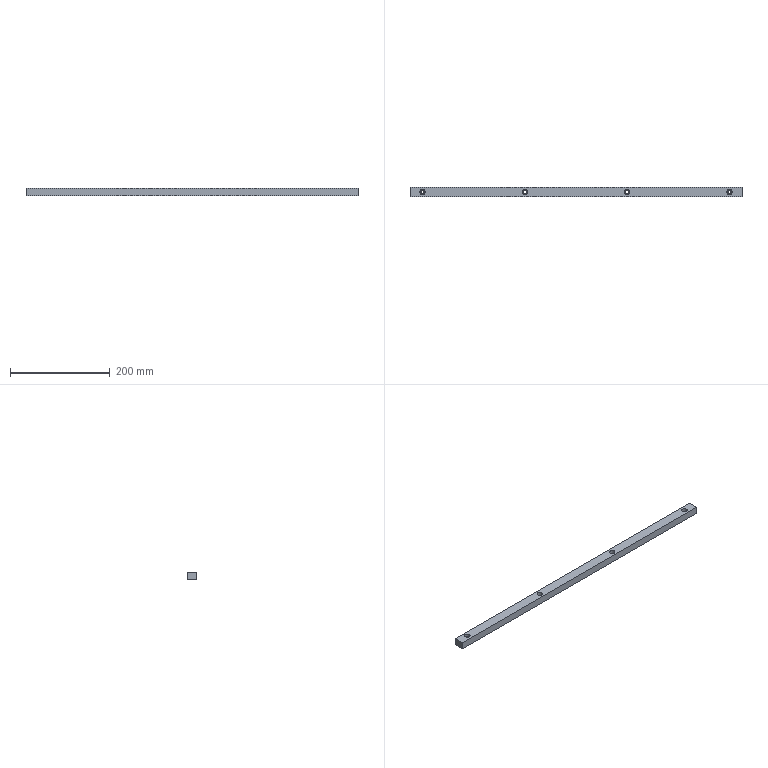Part | SolidWorks | features Extrusion 1, HoleWzd 1 | 1 solid | 26 faces | box 665 x 20 x 15 mm | volume 195793 mm3 | cylinder 16 | plane 10 | commonest cylinder face diameters 6.6 x8 11 x8
STEP:
#1=CARTESIAN_POINT('',(-313.,0.,8.2));
#2=VERTEX_POINT('',#1);
#3=CARTESIAN_POINT('',(-302.,0.,8.2));
#4=VERTEX_POINT('',#3);
#5=CARTESIAN_POINT('',(-307.5,0.,8.2));
#6=DIRECTION('',(0.,0.,1.));
#7=DIRECTION('',(1.,0.,0.));
#8=AXIS2_PLACEMENT_3D('',#5,#6,#7);
#9=CIRCLE('',#8,5.5);
#10=EDGE_CURVE('',#2,#4,#9,.T.);
#11=ORIENTED_EDGE('',*,*,#10,.F.);
#12=CARTESIAN_POINT('',(-313.,0.,15.));
#13=VERTEX_POINT('',#12);
#14=CARTESIAN_POINT('',(-313.,0.,15.));
#15=DIRECTION('',(0.,0.,1.));
#16=VECTOR('',#15,1000.);
#17=LINE('',#14,#16);
#18=EDGE_CURVE('',#2,#13,#17,.T.);
#19=ORIENTED_EDGE('',*,*,#18,.T.);
#20=CARTESIAN_POINT('',(-302.,0.,15.));
#21=VERTEX_POINT('',#20);
#22=CARTESIAN_POINT('',(-307.5,0.,15.));
#23=DIRECTION('',(0.,0.,1.));
#24=DIRECTION('',(1.,0.,0.));
#25=AXIS2_PLACEMENT_3D('',#22,#23,#24);
#26=CIRCLE('',#25,5.5);
#27=EDGE_CURVE('',#13,#21,#26,.T.);
#28=ORIENTED_EDGE('',*,*,#27,.T.);
#29=CARTESIAN_POINT('',(-302.,0.,15.));
#30=DIRECTION('',(0.,0.,1.));
#31=VECTOR('',#30,1000.);
#32=LINE('',#29,#31);
#33=EDGE_CURVE('',#4,#21,#32,.T.);
#34=ORIENTED_EDGE('',*,*,#33,.F.);
#35=EDGE_LOOP('',(#11,#19,#28,#34));
#36=FACE_OUTER_BOUND('',#35,.T.);
#37=CARTESIAN_POINT('',(-307.5,0.,15.));
#38=DIRECTION('',(0.,0.,1.));
#39=DIRECTION('',(1.,0.,0.));
#40=AXIS2_PLACEMENT_3D('',#37,#38,#39);
#41=CYLINDRICAL_SURFACE('',#40,5.5);
#42=ADVANCED_FACE('',(#36),#41,.F.);
#43=CARTESIAN_POINT('',(-310.8,0.,0.));
#44=VERTEX_POINT('',#43);
#45=CARTESIAN_POINT('',(-304.2,0.,0.));
#46=VERTEX_POINT('',#45);
#47=CARTESIAN_POINT('',(-307.5,0.,0.));
#48=DIRECTION('',(0.,0.,1.));
#49=DIRECTION('',(1.,0.,0.));
#50=AXIS2_PLACEMENT_3D('',#47,#48,#49);
#51=CIRCLE('',#50,3.3);
#52=EDGE_CURVE('',#44,#46,#51,.T.);
#53=ORIENTED_EDGE('',*,*,#52,.F.);
#54=CARTESIAN_POINT('',(-310.8,0.,8.2));
#55=VERTEX_POINT('',#54);
#56=CARTESIAN_POINT('',(-310.8,0.,15.));
#57=DIRECTION('',(0.,0.,1.));
#58=VECTOR('',#57,1000.);
#59=LINE('',#56,#58);
#60=EDGE_CURVE('',#44,#55,#59,.T.);
#61=ORIENTED_EDGE('',*,*,#60,.T.);
#62=CARTESIAN_POINT('',(-304.2,0.,8.2));
#63=VERTEX_POINT('',#62);
#64=CARTESIAN_POINT('',(-307.5,0.,8.2));
#65=DIRECTION('',(0.,0.,1.));
#66=DIRECTION('',(1.,0.,0.));
#67=AXIS2_PLACEMENT_3D('',#64,#65,#66);
#68=CIRCLE('',#67,3.3);
#69=EDGE_CURVE('',#55,#63,#68,.T.);
#70=ORIENTED_EDGE('',*,*,#69,.T.);
#71=CARTESIAN_POINT('',(-304.2,0.,15.));
#72=DIRECTION('',(0.,0.,1.));
#73=VECTOR('',#72,1000.);
#74=LINE('',#71,#73);
#75=EDGE_CURVE('',#46,#63,#74,.T.);
#76=ORIENTED_EDGE('',*,*,#75,.F.);
#77=EDGE_LOOP('',(#53,#61,#70,#76));
#78=FACE_OUTER_BOUND('',#77,.T.);
#79=CARTESIAN_POINT('',(-307.5,0.,15.));
#80=DIRECTION('',(0.,0.,1.));
#81=DIRECTION('',(1.,0.,0.));
#82=AXIS2_PLACEMENT_3D('',#79,#80,#81);
#83=CYLINDRICAL_SURFACE('',#82,3.3);
#84=ADVANCED_FACE('',(#78),#83,.F.);
#85=CARTESIAN_POINT('',(302.,0.,8.2));
#86=VERTEX_POINT('',#85);
#87=CARTESIAN_POINT('',(313.,0.,8.2));
#88=VERTEX_POINT('',#87);
#89=CARTESIAN_POINT('',(307.5,0.,8.2));
#90=DIRECTION('',(0.,0.,1.));
#91=DIRECTION('',(1.,0.,0.));
#92=AXIS2_PLACEMENT_3D('',#89,#90,#91);
#93=CIRCLE('',#92,5.5);
#94=EDGE_CURVE('',#86,#88,#93,.T.);
#95=ORIENTED_EDGE('',*,*,#94,.F.);
#96=CARTESIAN_POINT('',(302.,0.,15.));
#97=VERTEX_POINT('',#96);
#98=CARTESIAN_POINT('',(302.,0.,15.));
#99=DIRECTION('',(0.,0.,1.));
#100=VECTOR('',#99,1000.);
#101=LINE('',#98,#100);
#102=EDGE_CURVE('',#86,#97,#101,.T.);
#103=ORIENTED_EDGE('',*,*,#102,.T.);
#104=CARTESIAN_POINT('',(313.,0.,15.));
#105=VERTEX_POINT('',#104);
#106=CARTESIAN_POINT('',(307.5,0.,15.));
#107=DIRECTION('',(0.,0.,1.));
#108=DIRECTION('',(1.,0.,0.));
#109=AXIS2_PLACEMENT_3D('',#106,#107,#108);
#110=CIRCLE('',#109,5.5);
#111=EDGE_CURVE('',#97,#105,#110,.T.);
#112=ORIENTED_EDGE('',*,*,#111,.T.);
#113=CARTESIAN_POINT('',(313.,0.,15.));
#114=DIRECTION('',(0.,0.,1.));
#115=VECTOR('',#114,1000.);
#116=LINE('',#113,#115);
#117=EDGE_CURVE('',#88,#105,#116,.T.);
#118=ORIENTED_EDGE('',*,*,#117,.F.);
#119=EDGE_LOOP('',(#95,#103,#112,#118));
#120=FACE_OUTER_BOUND('',#119,.T.);
#121=CARTESIAN_POINT('',(307.5,0.,15.));
#122=DIRECTION('',(0.,0.,1.));
#123=DIRECTION('',(1.,0.,0.));
#124=AXIS2_PLACEMENT_3D('',#121,#122,#123);
#125=CYLINDRICAL_SURFACE('',#124,5.5);
#126=ADVANCED_FACE('',(#120),#125,.F.);
#127=CARTESIAN_POINT('',(304.2,0.,0.));
#128=VERTEX_POINT('',#127);
#129=CARTESIAN_POINT('',(310.8,0.,0.));
#130=VERTEX_POINT('',#129);
#131=CARTESIAN_POINT('',(307.5,0.,0.));
#132=DIRECTION('',(0.,0.,1.));
#133=DIRECTION('',(1.,0.,0.));
#134=AXIS2_PLACEMENT_3D('',#131,#132,#133);
#135=CIRCLE('',#134,3.3);
#136=EDGE_CURVE('',#128,#130,#135,.T.);
#137=ORIENTED_EDGE('',*,*,#136,.F.);
#138=CARTESIAN_POINT('',(304.2,0.,8.2));
#139=VERTEX_POINT('',#138);
#140=CARTESIAN_POINT('',(304.2,0.,15.));
#141=DIRECTION('',(0.,0.,1.));
#142=VECTOR('',#141,1000.);
#143=LINE('',#140,#142);
#144=EDGE_CURVE('',#128,#139,#143,.T.);
#145=ORIENTED_EDGE('',*,*,#144,.T.);
#146=CARTESIAN_POINT('',(310.8,0.,8.2));
#147=VERTEX_POINT('',#146);
#148=CARTESIAN_POINT('',(307.5,0.,8.2));
#149=DIRECTION('',(0.,0.,1.));
#150=DIRECTION('',(1.,0.,0.));
#151=AXIS2_PLACEMENT_3D('',#148,#149,#150);
#152=CIRCLE('',#151,3.3);
#153=EDGE_CURVE('',#139,#147,#152,.T.);
#154=ORIENTED_EDGE('',*,*,#153,.T.);
#155=CARTESIAN_POINT('',(310.8,0.,15.));
#156=DIRECTION('',(0.,0.,1.));
#157=VECTOR('',#156,1000.);
#158=LINE('',#155,#157);
#159=EDGE_CURVE('',#130,#147,#158,.T.);
#160=ORIENTED_EDGE('',*,*,#159,.F.);
#161=EDGE_LOOP('',(#137,#145,#154,#160));
#162=FACE_OUTER_BOUND('',#161,.T.);
#163=CARTESIAN_POINT('',(307.5,0.,15.));
#164=DIRECTION('',(0.,0.,1.));
#165=DIRECTION('',(1.,0.,0.));
#166=AXIS2_PLACEMENT_3D('',#163,#164,#165);
#167=CYLINDRICAL_SURFACE('',#166,3.3);
#168=ADVANCED_FACE('',(#162),#167,.F.);
#169=CARTESIAN_POINT('',(-108.,0.,8.2));
#170=VERTEX_POINT('',#169);
#171=CARTESIAN_POINT('',(-97.,0.,8.2));
#172=VERTEX_POINT('',#171);
#173=CARTESIAN_POINT('',(-102.5,0.,8.2));
#174=DIRECTION('',(0.,0.,1.));
#175=DIRECTION('',(1.,0.,0.));
#176=AXIS2_PLACEMENT_3D('',#173,#174,#175);
#177=CIRCLE('',#176,5.5);
#178=EDGE_CURVE('',#170,#172,#177,.T.);
#179=ORIENTED_EDGE('',*,*,#178,.F.);
#180=CARTESIAN_POINT('',(-108.,0.,15.));
#181=VERTEX_POINT('',#180);
#182=CARTESIAN_POINT('',(-108.,0.,15.));
#183=DIRECTION('',(0.,0.,1.));
#184=VECTOR('',#183,1000.);
#185=LINE('',#182,#184);
#186=EDGE_CURVE('',#170,#181,#185,.T.);
#187=ORIENTED_EDGE('',*,*,#186,.T.);
#188=CARTESIAN_POINT('',(-97.,0.,15.));
#189=VERTEX_POINT('',#188);
#190=CARTESIAN_POINT('',(-102.5,0.,15.));
#191=DIRECTION('',(0.,0.,1.));
#192=DIRECTION('',(1.,0.,0.));
#193=AXIS2_PLACEMENT_3D('',#190,#191,#192);
#194=CIRCLE('',#193,5.5);
#195=EDGE_CURVE('',#181,#189,#194,.T.);
#196=ORIENTED_EDGE('',*,*,#195,.T.);
#197=CARTESIAN_POINT('',(-97.,0.,15.));
#198=DIRECTION('',(0.,0.,1.));
#199=VECTOR('',#198,1000.);
#200=LINE('',#197,#199);
#201=EDGE_CURVE('',#172,#189,#200,.T.);
#202=ORIENTED_EDGE('',*,*,#201,.F.);
#203=EDGE_LOOP('',(#179,#187,#196,#202));
#204=FACE_OUTER_BOUND('',#203,.T.);
#205=CARTESIAN_POINT('',(-102.5,0.,15.));
#206=DIRECTION('',(0.,0.,1.));
#207=DIRECTION('',(1.,0.,0.));
#208=AXIS2_PLACEMENT_3D('',#205,#206,#207);
#209=CYLINDRICAL_SURFACE('',#208,5.5);
#210=ADVANCED_FACE('',(#204),#209,.F.);
#211=CARTESIAN_POINT('',(-105.8,0.,0.));
#212=VERTEX_POINT('',#211);
#213=CARTESIAN_POINT('',(-99.2,0.,0.));
#214=VERTEX_POINT('',#213);
#215=CARTESIAN_POINT('',(-102.5,0.,0.));
#216=DIRECTION('',(0.,0.,1.));
#217=DIRECTION('',(1.,0.,0.));
#218=AXIS2_PLACEMENT_3D('',#215,#216,#217);
#219=CIRCLE('',#218,3.3);
#220=EDGE_CURVE('',#212,#214,#219,.T.);
#221=ORIENTED_EDGE('',*,*,#220,.F.);
#222=CARTESIAN_POINT('',(-105.8,0.,8.2));
#223=VERTEX_POINT('',#222);
#224=CARTESIAN_POINT('',(-105.8,0.,15.));
#225=DIRECTION('',(0.,0.,1.));
#226=VECTOR('',#225,1000.);
#227=LINE('',#224,#226);
#228=EDGE_CURVE('',#212,#223,#227,.T.);
#229=ORIENTED_EDGE('',*,*,#228,.T.);
#230=CARTESIAN_POINT('',(-99.2,0.,8.2));
#231=VERTEX_POINT('',#230);
#232=CARTESIAN_POINT('',(-102.5,0.,8.2));
#233=DIRECTION('',(0.,0.,1.));
#234=DIRECTION('',(1.,0.,0.));
#235=AXIS2_PLACEMENT_3D('',#232,#233,#234);
#236=CIRCLE('',#235,3.3);
#237=EDGE_CURVE('',#223,#231,#236,.T.);
#238=ORIENTED_EDGE('',*,*,#237,.T.);
#239=CARTESIAN_POINT('',(-99.2,0.,15.));
#240=DIRECTION('',(0.,0.,1.));
#241=VECTOR('',#240,1000.);
#242=LINE('',#239,#241);
#243=EDGE_CURVE('',#214,#231,#242,.T.);
#244=ORIENTED_EDGE('',*,*,#243,.F.);
#245=EDGE_LOOP('',(#221,#229,#238,#244));
#246=FACE_OUTER_BOUND('',#245,.T.);
#247=CARTESIAN_POINT('',(-102.5,0.,15.));
#248=DIRECTION('',(0.,0.,1.));
#249=DIRECTION('',(1.,0.,0.));
#250=AXIS2_PLACEMENT_3D('',#247,#248,#249);
#251=CYLINDRICAL_SURFACE('',#250,3.3);
#252=ADVANCED_FACE('',(#246),#251,.F.);
#253=CARTESIAN_POINT('',(97.,0.,8.2));
#254=VERTEX_POINT('',#253);
#255=CARTESIAN_POINT('',(108.,0.,8.2));
#256=VERTEX_POINT('',#255);
#257=CARTESIAN_POINT('',(102.5,0.,8.2));
#258=DIRECTION('',(0.,0.,1.));
#259=DIRECTION('',(1.,0.,0.));
#260=AXIS2_PLACEMENT_3D('',#257,#258,#259);
#261=CIRCLE('',#260,5.5);
#262=EDGE_CURVE('',#254,#256,#261,.T.);
#263=ORIENTED_EDGE('',*,*,#262,.F.);
#264=CARTESIAN_POINT('',(97.,0.,15.));
#265=VERTEX_POINT('',#264);
#266=CARTESIAN_POINT('',(97.,0.,15.));
#267=DIRECTION('',(0.,0.,1.));
#268=VECTOR('',#267,1000.);
#269=LINE('',#266,#268);
#270=EDGE_CURVE('',#254,#265,#269,.T.);
#271=ORIENTED_EDGE('',*,*,#270,.T.);
#272=CARTESIAN_POINT('',(108.,0.,15.));
#273=VERTEX_POINT('',#272);
#274=CARTESIAN_POINT('',(102.5,0.,15.));
#275=DIRECTION('',(0.,0.,1.));
#276=DIRECTION('',(1.,0.,0.));
#277=AXIS2_PLACEMENT_3D('',#274,#275,#276);
#278=CIRCLE('',#277,5.5);
#279=EDGE_CURVE('',#265,#273,#278,.T.);
#280=ORIENTED_EDGE('',*,*,#279,.T.);
#281=CARTESIAN_POINT('',(108.,0.,15.));
#282=DIRECTION('',(0.,0.,1.));
#283=VECTOR('',#282,1000.);
#284=LINE('',#281,#283);
#285=EDGE_CURVE('',#256,#273,#284,.T.);
#286=ORIENTED_EDGE('',*,*,#285,.F.);
#287=EDGE_LOOP('',(#263,#271,#280,#286));
#288=FACE_OUTER_BOUND('',#287,.T.);
#289=CARTESIAN_POINT('',(102.5,0.,15.));
#290=DIRECTION('',(0.,0.,1.));
#291=DIRECTION('',(1.,0.,0.));
#292=AXIS2_PLACEMENT_3D('',#289,#290,#291);
#293=CYLINDRICAL_SURFACE('',#292,5.5);
#294=ADVANCED_FACE('',(#288),#293,.F.);
#295=CARTESIAN_POINT('',(99.2,0.,0.));
#296=VERTEX_POINT('',#295);
#297=CARTESIAN_POINT('',(105.8,0.,0.));
#298=VERTEX_POINT('',#297);
#299=CARTESIAN_POINT('',(102.5,0.,0.));
#300=DIRECTION('',(0.,0.,1.));
#301=DIRECTION('',(1.,0.,0.));
#302=AXIS2_PLACEMENT_3D('',#299,#300,#301);
#303=CIRCLE('',#302,3.3);
#304=EDGE_CURVE('',#296,#298,#303,.T.);
#305=ORIENTED_EDGE('',*,*,#304,.F.);
#306=CARTESIAN_POINT('',(99.2,0.,8.2));
#307=VERTEX_POINT('',#306);
#308=CARTESIAN_POINT('',(99.2,0.,15.));
#309=DIRECTION('',(0.,0.,1.));
#310=VECTOR('',#309,1000.);
#311=LINE('',#308,#310);
#312=EDGE_CURVE('',#296,#307,#311,.T.);
#313=ORIENTED_EDGE('',*,*,#312,.T.);
#314=CARTESIAN_POINT('',(105.8,0.,8.2));
#315=VERTEX_POINT('',#314);
#316=CARTESIAN_POINT('',(102.5,0.,8.2));
#317=DIRECTION('',(0.,0.,1.));
#318=DIRECTION('',(1.,0.,0.));
#319=AXIS2_PLACEMENT_3D('',#316,#317,#318);
#320=CIRCLE('',#319,3.3);
#321=EDGE_CURVE('',#307,#315,#320,.T.);
#322=ORIENTED_EDGE('',*,*,#321,.T.);
#323=CARTESIAN_POINT('',(105.8,0.,15.));
#324=DIRECTION('',(0.,0.,1.));
#325=VECTOR('',#324,1000.);
#326=LINE('',#323,#325);
#327=EDGE_CURVE('',#298,#315,#326,.T.);
#328=ORIENTED_EDGE('',*,*,#327,.F.);
#329=EDGE_LOOP('',(#305,#313,#322,#328));
#330=FACE_OUTER_BOUND('',#329,.T.);
#331=CARTESIAN_POINT('',(102.5,0.,15.));
#332=DIRECTION('',(0.,0.,1.));
#333=DIRECTION('',(1.,0.,0.));
#334=AXIS2_PLACEMENT_3D('',#331,#332,#333);
#335=CYLINDRICAL_SURFACE('',#334,3.3);
#336=ADVANCED_FACE('',(#330),#335,.F.);
#337=CARTESIAN_POINT('',(332.5,-10.,0.));
#338=VERTEX_POINT('',#337);
#339=CARTESIAN_POINT('',(332.5,10.,0.));
#340=VERTEX_POINT('',#339);
#341=CARTESIAN_POINT('',(332.5,10.,0.));
#342=DIRECTION('',(0.,1.,0.));
#343=VECTOR('',#342,1000.);
#344=LINE('',#341,#343);
#345=EDGE_CURVE('',#338,#340,#344,.T.);
#346=ORIENTED_EDGE('',*,*,#345,.T.);
#347=CARTESIAN_POINT('',(332.5,10.,15.));
#348=VERTEX_POINT('',#347);
#349=CARTESIAN_POINT('',(332.5,10.,15.));
#350=DIRECTION('',(0.,0.,-1.));
#351=VECTOR('',#350,1000.);
#352=LINE('',#349,#351);
#353=EDGE_CURVE('',#348,#340,#352,.T.);
#354=ORIENTED_EDGE('',*,*,#353,.F.);
#355=CARTESIAN_POINT('',(332.5,-10.,15.));
#356=VERTEX_POINT('',#355);
#357=CARTESIAN_POINT('',(332.5,10.,15.));
#358=DIRECTION('',(0.,1.,0.));
#359=VECTOR('',#358,1000.);
#360=LINE('',#357,#359);
#361=EDGE_CURVE('',#356,#348,#360,.T.);
#362=ORIENTED_EDGE('',*,*,#361,.F.);
#363=CARTESIAN_POINT('',(332.5,-10.,15.));
#364=DIRECTION('',(0.,0.,-1.));
#365=VECTOR('',#364,1000.);
#366=LINE('',#363,#365);
#367=EDGE_CURVE('',#356,#338,#366,.T.);
#368=ORIENTED_EDGE('',*,*,#367,.T.);
#369=EDGE_LOOP('',(#346,#354,#362,#368));
#370=FACE_OUTER_BOUND('',#369,.T.);
#371=CARTESIAN_POINT('',(332.5,10.,15.));
#372=DIRECTION('',(-1.,0.,0.));
#373=DIRECTION('',(0.,0.,1.));
#374=AXIS2_PLACEMENT_3D('',#371,#372,#373);
#375=PLANE('',#374);
#376=ADVANCED_FACE('',(#370),#375,.F.);
#377=CARTESIAN_POINT('',(-332.5,10.,0.));
#378=VERTEX_POINT('',#377);
#379=CARTESIAN_POINT('',(-332.5,10.,0.));
#380=DIRECTION('',(-1.,0.,0.));
#381=VECTOR('',#380,1000.);
#382=LINE('',#379,#381);
#383=EDGE_CURVE('',#340,#378,#382,.T.);
#384=ORIENTED_EDGE('',*,*,#383,.T.);
#385=CARTESIAN_POINT('',(-332.5,10.,15.));
#386=VERTEX_POINT('',#385);
#387=CARTESIAN_POINT('',(-332.5,10.,15.));
#388=DIRECTION('',(0.,0.,-1.));
#389=VECTOR('',#388,1000.);
#390=LINE('',#387,#389);
#391=EDGE_CURVE('',#386,#378,#390,.T.);
#392=ORIENTED_EDGE('',*,*,#391,.F.);
#393=CARTESIAN_POINT('',(-332.5,10.,15.));
#394=DIRECTION('',(-1.,0.,0.));
#395=VECTOR('',#394,1000.);
#396=LINE('',#393,#395);
#397=EDGE_CURVE('',#348,#386,#396,.T.);
#398=ORIENTED_EDGE('',*,*,#397,.F.);
#399=ORIENTED_EDGE('',*,*,#353,.T.);
#400=EDGE_LOOP('',(#384,#392,#398,#399));
#401=FACE_OUTER_BOUND('',#400,.T.);
#402=CARTESIAN_POINT('',(-332.5,10.,15.));
#403=DIRECTION('',(0.,-1.,0.));
#404=DIRECTION('',(0.,0.,-1.));
#405=AXIS2_PLACEMENT_3D('',#402,#403,#404);
#406=PLANE('',#405);
#407=ADVANCED_FACE('',(#401),#406,.F.);
#408=CARTESIAN_POINT('',(-332.5,-10.,0.));
#409=VERTEX_POINT('',#408);
#410=CARTESIAN_POINT('',(-332.5,10.,0.));
#411=DIRECTION('',(0.,-1.,0.));
#412=VECTOR('',#411,1000.);
#413=LINE('',#410,#412);
#414=EDGE_CURVE('',#378,#409,#413,.T.);
#415=ORIENTED_EDGE('',*,*,#414,.T.);
#416=CARTESIAN_POINT('',(-332.5,-10.,15.));
#417=VERTEX_POINT('',#416);
#418=CARTESIAN_POINT('',(-332.5,-10.,15.));
#419=DIRECTION('',(0.,0.,-1.));
#420=VECTOR('',#419,1000.);
#421=LINE('',#418,#420);
#422=EDGE_CURVE('',#417,#409,#421,.T.);
#423=ORIENTED_EDGE('',*,*,#422,.F.);
#424=CARTESIAN_POINT('',(-332.5,10.,15.));
#425=DIRECTION('',(0.,-1.,0.));
#426=VECTOR('',#425,1000.);
#427=LINE('',#424,#426);
#428=EDGE_CURVE('',#386,#417,#427,.T.);
#429=ORIENTED_EDGE('',*,*,#428,.F.);
#430=ORIENTED_EDGE('',*,*,#391,.T.);
#431=EDGE_LOOP('',(#415,#423,#429,#430));
#432=FACE_OUTER_BOUND('',#431,.T.);
#433=CARTESIAN_POINT('',(-332.5,10.,15.));
#434=DIRECTION('',(1.,0.,0.));
#435=DIRECTION('',(0.,0.,-1.));
#436=AXIS2_PLACEMENT_3D('',#433,#434,#435);
#437=PLANE('',#436);
#438=ADVANCED_FACE('',(#432),#437,.F.);
#439=CARTESIAN_POINT('',(-332.5,-10.,0.));
#440=DIRECTION('',(1.,0.,0.));
#441=VECTOR('',#440,1000.);
#442=LINE('',#439,#441);
#443=EDGE_CURVE('',#409,#338,#442,.T.);
#444=ORIENTED_EDGE('',*,*,#443,.T.);
#445=ORIENTED_EDGE('',*,*,#367,.F.);
#446=CARTESIAN_POINT('',(-332.5,-10.,15.));
#447=DIRECTION('',(1.,0.,0.));
#448=VECTOR('',#447,1000.);
#449=LINE('',#446,#448);
#450=EDGE_CURVE('',#417,#356,#449,.T.);
#451=ORIENTED_EDGE('',*,*,#450,.F.);
#452=ORIENTED_EDGE('',*,*,#422,.T.);
#453=EDGE_LOOP('',(#444,#445,#451,#452));
#454=FACE_OUTER_BOUND('',#453,.T.);
#455=CARTESIAN_POINT('',(-332.5,-10.,15.));
#456=DIRECTION('',(0.,1.,0.));
#457=DIRECTION('',(0.,0.,1.));
#458=AXIS2_PLACEMENT_3D('',#455,#456,#457);
#459=PLANE('',#458);
#460=ADVANCED_FACE('',(#454),#459,.F.);
#461=CARTESIAN_POINT('',(-307.5,0.,15.));
#462=DIRECTION('',(0.,0.,1.));
#463=DIRECTION('',(1.,0.,0.));
#464=AXIS2_PLACEMENT_3D('',#461,#462,#463);
#465=CIRCLE('',#464,5.5);
#466=EDGE_CURVE('',#21,#13,#465,.T.);
#467=ORIENTED_EDGE('',*,*,#466,.F.);
#468=ORIENTED_EDGE('',*,*,#27,.F.);
#469=EDGE_LOOP('',(#467,#468));
#470=FACE_BOUND('',#469,.T.);
#471=CARTESIAN_POINT('',(307.5,0.,15.));
#472=DIRECTION('',(0.,0.,1.));
#473=DIRECTION('',(1.,0.,0.));
#474=AXIS2_PLACEMENT_3D('',#471,#472,#473);
#475=CIRCLE('',#474,5.5);
#476=EDGE_CURVE('',#105,#97,#475,.T.);
#477=ORIENTED_EDGE('',*,*,#476,.F.);
#478=ORIENTED_EDGE('',*,*,#111,.F.);
#479=EDGE_LOOP('',(#477,#478));
#480=FACE_BOUND('',#479,.T.);
#481=CARTESIAN_POINT('',(-102.5,0.,15.));
#482=DIRECTION('',(0.,0.,1.));
#483=DIRECTION('',(1.,0.,0.));
#484=AXIS2_PLACEMENT_3D('',#481,#482,#483);
#485=CIRCLE('',#484,5.5);
#486=EDGE_CURVE('',#189,#181,#485,.T.);
#487=ORIENTED_EDGE('',*,*,#486,.F.);
#488=ORIENTED_EDGE('',*,*,#195,.F.);
#489=EDGE_LOOP('',(#487,#488));
#490=FACE_BOUND('',#489,.T.);
#491=CARTESIAN_POINT('',(102.5,0.,15.));
#492=DIRECTION('',(0.,0.,1.));
#493=DIRECTION('',(1.,0.,0.));
#494=AXIS2_PLACEMENT_3D('',#491,#492,#493);
#495=CIRCLE('',#494,5.5);
#496=EDGE_CURVE('',#273,#265,#495,.T.);
#497=ORIENTED_EDGE('',*,*,#496,.F.);
#498=ORIENTED_EDGE('',*,*,#279,.F.);
#499=EDGE_LOOP('',(#497,#498));
#500=FACE_BOUND('',#499,.T.);
#501=ORIENTED_EDGE('',*,*,#361,.T.);
#502=ORIENTED_EDGE('',*,*,#397,.T.);
#503=ORIENTED_EDGE('',*,*,#428,.T.);
#504=ORIENTED_EDGE('',*,*,#450,.T.);
#505=EDGE_LOOP('',(#501,#502,#503,#504));
#506=FACE_OUTER_BOUND('',#505,.T.);
#507=CARTESIAN_POINT('',(0.,0.,15.));
#508=DIRECTION('',(0.,0.,1.));
#509=DIRECTION('',(1.,0.,0.));
#510=AXIS2_PLACEMENT_3D('',#507,#508,#509);
#511=PLANE('',#510);
#512=ADVANCED_FACE('',(#470,#480,#490,#500,#506),#511,.T.);
#513=CARTESIAN_POINT('',(-307.5,0.,0.));
#514=DIRECTION('',(0.,0.,1.));
#515=DIRECTION('',(1.,0.,0.));
#516=AXIS2_PLACEMENT_3D('',#513,#514,#515);
#517=CIRCLE('',#516,3.3);
#518=EDGE_CURVE('',#46,#44,#517,.T.);
#519=ORIENTED_EDGE('',*,*,#518,.T.);
#520=ORIENTED_EDGE('',*,*,#52,.T.);
#521=EDGE_LOOP('',(#519,#520));
#522=FACE_BOUND('',#521,.T.);
#523=CARTESIAN_POINT('',(307.5,0.,0.));
#524=DIRECTION('',(0.,0.,1.));
#525=DIRECTION('',(1.,0.,0.));
#526=AXIS2_PLACEMENT_3D('',#523,#524,#525);
#527=CIRCLE('',#526,3.3);
#528=EDGE_CURVE('',#130,#128,#527,.T.);
#529=ORIENTED_EDGE('',*,*,#528,.T.);
#530=ORIENTED_EDGE('',*,*,#136,.T.);
#531=EDGE_LOOP('',(#529,#530));
#532=FACE_BOUND('',#531,.T.);
#533=CARTESIAN_POINT('',(-102.5,0.,0.));
#534=DIRECTION('',(0.,0.,1.));
#535=DIRECTION('',(1.,0.,0.));
#536=AXIS2_PLACEMENT_3D('',#533,#534,#535);
#537=CIRCLE('',#536,3.3);
#538=EDGE_CURVE('',#214,#212,#537,.T.);
#539=ORIENTED_EDGE('',*,*,#538,.T.);
#540=ORIENTED_EDGE('',*,*,#220,.T.);
#541=EDGE_LOOP('',(#539,#540));
#542=FACE_BOUND('',#541,.T.);
#543=CARTESIAN_POINT('',(102.5,0.,0.));
#544=DIRECTION('',(0.,0.,1.));
#545=DIRECTION('',(1.,0.,0.));
#546=AXIS2_PLACEMENT_3D('',#543,#544,#545);
#547=CIRCLE('',#546,3.3);
#548=EDGE_CURVE('',#298,#296,#547,.T.);
#549=ORIENTED_EDGE('',*,*,#548,.T.);
#550=ORIENTED_EDGE('',*,*,#304,.T.);
#551=EDGE_LOOP('',(#549,#550));
#552=FACE_BOUND('',#551,.T.);
#553=ORIENTED_EDGE('',*,*,#345,.F.);
#554=ORIENTED_EDGE('',*,*,#443,.F.);
#555=ORIENTED_EDGE('',*,*,#414,.F.);
#556=ORIENTED_EDGE('',*,*,#383,.F.);
#557=EDGE_LOOP('',(#553,#554,#555,#556));
#558=FACE_OUTER_BOUND('',#557,.T.);
#559=CARTESIAN_POINT('',(0.,0.,0.));
#560=DIRECTION('',(0.,0.,1.));
#561=DIRECTION('',(1.,0.,0.));
#562=AXIS2_PLACEMENT_3D('',#559,#560,#561);
#563=PLANE('',#562);
#564=ADVANCED_FACE('',(#522,#532,#542,#552,#558),#563,.F.);
#565=ORIENTED_EDGE('',*,*,#312,.F.);
#566=ORIENTED_EDGE('',*,*,#548,.F.);
#567=ORIENTED_EDGE('',*,*,#327,.T.);
#568=CARTESIAN_POINT('',(102.5,0.,8.2));
#569=DIRECTION('',(0.,0.,1.));
#570=DIRECTION('',(1.,0.,0.));
#571=AXIS2_PLACEMENT_3D('',#568,#569,#570);
#572=CIRCLE('',#571,3.3);
#573=EDGE_CURVE('',#315,#307,#572,.T.);
#574=ORIENTED_EDGE('',*,*,#573,.T.);
#575=EDGE_LOOP('',(#565,#566,#567,#574));
#576=FACE_OUTER_BOUND('',#575,.T.);
#577=CARTESIAN_POINT('',(102.5,0.,15.));
#578=DIRECTION('',(0.,0.,1.));
#579=DIRECTION('',(1.,0.,0.));
#580=AXIS2_PLACEMENT_3D('',#577,#578,#579);
#581=CYLINDRICAL_SURFACE('',#580,3.3);
#582=ADVANCED_FACE('',(#576),#581,.F.);
#583=ORIENTED_EDGE('',*,*,#573,.F.);
#584=ORIENTED_EDGE('',*,*,#321,.F.);
#585=EDGE_LOOP('',(#583,#584));
#586=FACE_BOUND('',#585,.T.);
#587=CARTESIAN_POINT('',(102.5,0.,8.2));
#588=DIRECTION('',(0.,0.,1.));
#589=DIRECTION('',(1.,0.,0.));
#590=AXIS2_PLACEMENT_3D('',#587,#588,#589);
#591=CIRCLE('',#590,5.5);
#592=EDGE_CURVE('',#256,#254,#591,.T.);
#593=ORIENTED_EDGE('',*,*,#592,.T.);
#594=ORIENTED_EDGE('',*,*,#262,.T.);
#595=EDGE_LOOP('',(#593,#594));
#596=FACE_OUTER_BOUND('',#595,.T.);
#597=CARTESIAN_POINT('',(105.8,0.,8.2));
#598=DIRECTION('',(0.,0.,-1.));
#599=DIRECTION('',(-1.,0.,0.));
#600=AXIS2_PLACEMENT_3D('',#597,#598,#599);
#601=PLANE('',#600);
#602=ADVANCED_FACE('',(#586,#596),#601,.F.);
#603=ORIENTED_EDGE('',*,*,#270,.F.);
#604=ORIENTED_EDGE('',*,*,#592,.F.);
#605=ORIENTED_EDGE('',*,*,#285,.T.);
#606=ORIENTED_EDGE('',*,*,#496,.T.);
#607=EDGE_LOOP('',(#603,#604,#605,#606));
#608=FACE_OUTER_BOUND('',#607,.T.);
#609=CARTESIAN_POINT('',(102.5,0.,15.));
#610=DIRECTION('',(0.,0.,1.));
#611=DIRECTION('',(1.,0.,0.));
#612=AXIS2_PLACEMENT_3D('',#609,#610,#611);
#613=CYLINDRICAL_SURFACE('',#612,5.5);
#614=ADVANCED_FACE('',(#608),#613,.F.);
#615=ORIENTED_EDGE('',*,*,#228,.F.);
#616=ORIENTED_EDGE('',*,*,#538,.F.);
#617=ORIENTED_EDGE('',*,*,#243,.T.);
#618=CARTESIAN_POINT('',(-102.5,0.,8.2));
#619=DIRECTION('',(0.,0.,1.));
#620=DIRECTION('',(1.,0.,0.));
#621=AXIS2_PLACEMENT_3D('',#618,#619,#620);
#622=CIRCLE('',#621,3.3);
#623=EDGE_CURVE('',#231,#223,#622,.T.);
#624=ORIENTED_EDGE('',*,*,#623,.T.);
#625=EDGE_LOOP('',(#615,#616,#617,#624));
#626=FACE_OUTER_BOUND('',#625,.T.);
#627=CARTESIAN_POINT('',(-102.5,0.,15.));
#628=DIRECTION('',(0.,0.,1.));
#629=DIRECTION('',(1.,0.,0.));
#630=AXIS2_PLACEMENT_3D('',#627,#628,#629);
#631=CYLINDRICAL_SURFACE('',#630,3.3);
#632=ADVANCED_FACE('',(#626),#631,.F.);
#633=ORIENTED_EDGE('',*,*,#623,.F.);
#634=ORIENTED_EDGE('',*,*,#237,.F.);
#635=EDGE_LOOP('',(#633,#634));
#636=FACE_BOUND('',#635,.T.);
#637=CARTESIAN_POINT('',(-102.5,0.,8.2));
#638=DIRECTION('',(0.,0.,1.));
#639=DIRECTION('',(1.,0.,0.));
#640=AXIS2_PLACEMENT_3D('',#637,#638,#639);
#641=CIRCLE('',#640,5.5);
#642=EDGE_CURVE('',#172,#170,#641,.T.);
#643=ORIENTED_EDGE('',*,*,#642,.T.);
#644=ORIENTED_EDGE('',*,*,#178,.T.);
#645=EDGE_LOOP('',(#643,#644));
#646=FACE_OUTER_BOUND('',#645,.T.);
#647=CARTESIAN_POINT('',(-99.2,0.,8.2));
#648=DIRECTION('',(0.,0.,-1.));
#649=DIRECTION('',(-1.,0.,0.));
#650=AXIS2_PLACEMENT_3D('',#647,#648,#649);
#651=PLANE('',#650);
#652=ADVANCED_FACE('',(#636,#646),#651,.F.);
#653=ORIENTED_EDGE('',*,*,#186,.F.);
#654=ORIENTED_EDGE('',*,*,#642,.F.);
#655=ORIENTED_EDGE('',*,*,#201,.T.);
#656=ORIENTED_EDGE('',*,*,#486,.T.);
#657=EDGE_LOOP('',(#653,#654,#655,#656));
#658=FACE_OUTER_BOUND('',#657,.T.);
#659=CARTESIAN_POINT('',(-102.5,0.,15.));
#660=DIRECTION('',(0.,0.,1.));
#661=DIRECTION('',(1.,0.,0.));
#662=AXIS2_PLACEMENT_3D('',#659,#660,#661);
#663=CYLINDRICAL_SURFACE('',#662,5.5);
#664=ADVANCED_FACE('',(#658),#663,.F.);
#665=ORIENTED_EDGE('',*,*,#144,.F.);
#666=ORIENTED_EDGE('',*,*,#528,.F.);
#667=ORIENTED_EDGE('',*,*,#159,.T.);
#668=CARTESIAN_POINT('',(307.5,0.,8.2));
#669=DIRECTION('',(0.,0.,1.));
#670=DIRECTION('',(1.,0.,0.));
#671=AXIS2_PLACEMENT_3D('',#668,#669,#670);
#672=CIRCLE('',#671,3.3);
#673=EDGE_CURVE('',#147,#139,#672,.T.);
#674=ORIENTED_EDGE('',*,*,#673,.T.);
#675=EDGE_LOOP('',(#665,#666,#667,#674));
#676=FACE_OUTER_BOUND('',#675,.T.);
#677=CARTESIAN_POINT('',(307.5,0.,15.));
#678=DIRECTION('',(0.,0.,1.));
#679=DIRECTION('',(1.,0.,0.));
#680=AXIS2_PLACEMENT_3D('',#677,#678,#679);
#681=CYLINDRICAL_SURFACE('',#680,3.3);
#682=ADVANCED_FACE('',(#676),#681,.F.);
#683=ORIENTED_EDGE('',*,*,#673,.F.);
#684=ORIENTED_EDGE('',*,*,#153,.F.);
#685=EDGE_LOOP('',(#683,#684));
#686=FACE_BOUND('',#685,.T.);
#687=CARTESIAN_POINT('',(307.5,0.,8.2));
#688=DIRECTION('',(0.,0.,1.));
#689=DIRECTION('',(1.,0.,0.));
#690=AXIS2_PLACEMENT_3D('',#687,#688,#689);
#691=CIRCLE('',#690,5.5);
#692=EDGE_CURVE('',#88,#86,#691,.T.);
#693=ORIENTED_EDGE('',*,*,#692,.T.);
#694=ORIENTED_EDGE('',*,*,#94,.T.);
#695=EDGE_LOOP('',(#693,#694));
#696=FACE_OUTER_BOUND('',#695,.T.);
#697=CARTESIAN_POINT('',(310.8,0.,8.2));
#698=DIRECTION('',(0.,0.,-1.));
#699=DIRECTION('',(-1.,0.,0.));
#700=AXIS2_PLACEMENT_3D('',#697,#698,#699);
#701=PLANE('',#700);
#702=ADVANCED_FACE('',(#686,#696),#701,.F.);
#703=ORIENTED_EDGE('',*,*,#102,.F.);
#704=ORIENTED_EDGE('',*,*,#692,.F.);
#705=ORIENTED_EDGE('',*,*,#117,.T.);
#706=ORIENTED_EDGE('',*,*,#476,.T.);
#707=EDGE_LOOP('',(#703,#704,#705,#706));
#708=FACE_OUTER_BOUND('',#707,.T.);
#709=CARTESIAN_POINT('',(307.5,0.,15.));
#710=DIRECTION('',(0.,0.,1.));
#711=DIRECTION('',(1.,0.,0.));
#712=AXIS2_PLACEMENT_3D('',#709,#710,#711);
#713=CYLINDRICAL_SURFACE('',#712,5.5);
#714=ADVANCED_FACE('',(#708),#713,.F.);
#715=ORIENTED_EDGE('',*,*,#60,.F.);
#716=ORIENTED_EDGE('',*,*,#518,.F.);
#717=ORIENTED_EDGE('',*,*,#75,.T.);
#718=CARTESIAN_POINT('',(-307.5,0.,8.2));
#719=DIRECTION('',(0.,0.,1.));
#720=DIRECTION('',(1.,0.,0.));
#721=AXIS2_PLACEMENT_3D('',#718,#719,#720);
#722=CIRCLE('',#721,3.3);
#723=EDGE_CURVE('',#63,#55,#722,.T.);
#724=ORIENTED_EDGE('',*,*,#723,.T.);
#725=EDGE_LOOP('',(#715,#716,#717,#724));
#726=FACE_OUTER_BOUND('',#725,.T.);
#727=CARTESIAN_POINT('',(-307.5,0.,15.));
#728=DIRECTION('',(0.,0.,1.));
#729=DIRECTION('',(1.,0.,0.));
#730=AXIS2_PLACEMENT_3D('',#727,#728,#729);
#731=CYLINDRICAL_SURFACE('',#730,3.3);
#732=ADVANCED_FACE('',(#726),#731,.F.);
#733=ORIENTED_EDGE('',*,*,#723,.F.);
#734=ORIENTED_EDGE('',*,*,#69,.F.);
#735=EDGE_LOOP('',(#733,#734));
#736=FACE_BOUND('',#735,.T.);
#737=CARTESIAN_POINT('',(-307.5,0.,8.2));
#738=DIRECTION('',(0.,0.,1.));
#739=DIRECTION('',(1.,0.,0.));
#740=AXIS2_PLACEMENT_3D('',#737,#738,#739);
#741=CIRCLE('',#740,5.5);
#742=EDGE_CURVE('',#4,#2,#741,.T.);
#743=ORIENTED_EDGE('',*,*,#742,.T.);
#744=ORIENTED_EDGE('',*,*,#10,.T.);
#745=EDGE_LOOP('',(#743,#744));
#746=FACE_OUTER_BOUND('',#745,.T.);
#747=CARTESIAN_POINT('',(-304.2,0.,8.2));
#748=DIRECTION('',(0.,0.,-1.));
#749=DIRECTION('',(-1.,0.,0.));
#750=AXIS2_PLACEMENT_3D('',#747,#748,#749);
#751=PLANE('',#750);
#752=ADVANCED_FACE('',(#736,#746),#751,.F.);
#753=ORIENTED_EDGE('',*,*,#18,.F.);
#754=ORIENTED_EDGE('',*,*,#742,.F.);
#755=ORIENTED_EDGE('',*,*,#33,.T.);
#756=ORIENTED_EDGE('',*,*,#466,.T.);
#757=EDGE_LOOP('',(#753,#754,#755,#756));
#758=FACE_OUTER_BOUND('',#757,.T.);
#759=CARTESIAN_POINT('',(-307.5,0.,15.));
#760=DIRECTION('',(0.,0.,1.));
#761=DIRECTION('',(1.,0.,0.));
#762=AXIS2_PLACEMENT_3D('',#759,#760,#761);
#763=CYLINDRICAL_SURFACE('',#762,5.5);
#764=ADVANCED_FACE('',(#758),#763,.F.);
#765=CLOSED_SHELL('',(#42,#84,#126,#168,#210,#252,#294,#336,#376,#407,#438,#460,#512,#564,#582,#602,#614,#632,#652,#664,#682,#702,#714,#732,#752,#764));
#766=MANIFOLD_SOLID_BREP('',#765);
#767=CARTESIAN_POINT('',(0.,0.,0.));
#768=DIRECTION('',(0.,0.,1.));
#769=DIRECTION('',(1.,0.,0.));
#770=AXIS2_PLACEMENT_3D('',#767,#768,#769);
#771=(LENGTH_UNIT()NAMED_UNIT(*)SI_UNIT(.MILLI.,.METRE.));
#772=UNCERTAINTY_MEASURE_WITH_UNIT(LENGTH_MEASURE(0.00001),#771,'','');
#773=(NAMED_UNIT(*)PLANE_ANGLE_UNIT()SI_UNIT($,.RADIAN.));
#774=(NAMED_UNIT(*)SI_UNIT($,.STERADIAN.)SOLID_ANGLE_UNIT());
#775=(GEOMETRIC_REPRESENTATION_CONTEXT(3)GLOBAL_UNCERTAINTY_ASSIGNED_CONTEXT((#772))GLOBAL_UNIT_ASSIGNED_CONTEXT((#771,#773,#774))REPRESENTATION_CONTEXT('',''));
#776=ADVANCED_BREP_SHAPE_REPRESENTATION('',(#766,#770),#775);